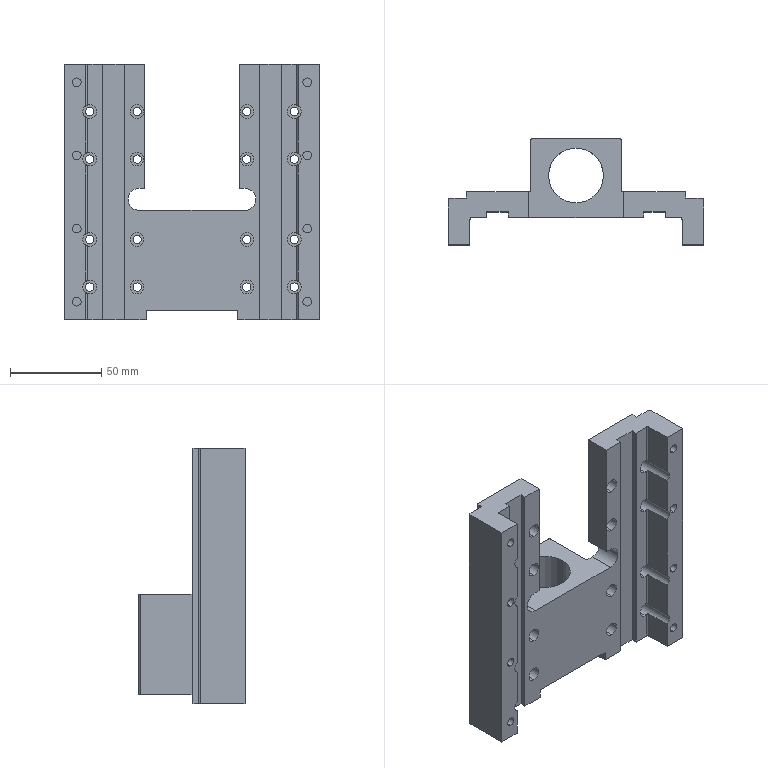Part | STEP file | SM140A-20-1140D-Side slide plate | 1 solid | 169 faces | box 140 x 58 x 140 mm | volume 271598 mm3 | cylinder 101 | plane 68 | commonest cylinder face diameters 4.5 x32 7.5 x32 2 x16 4.8 x16 12 x3 30 x2